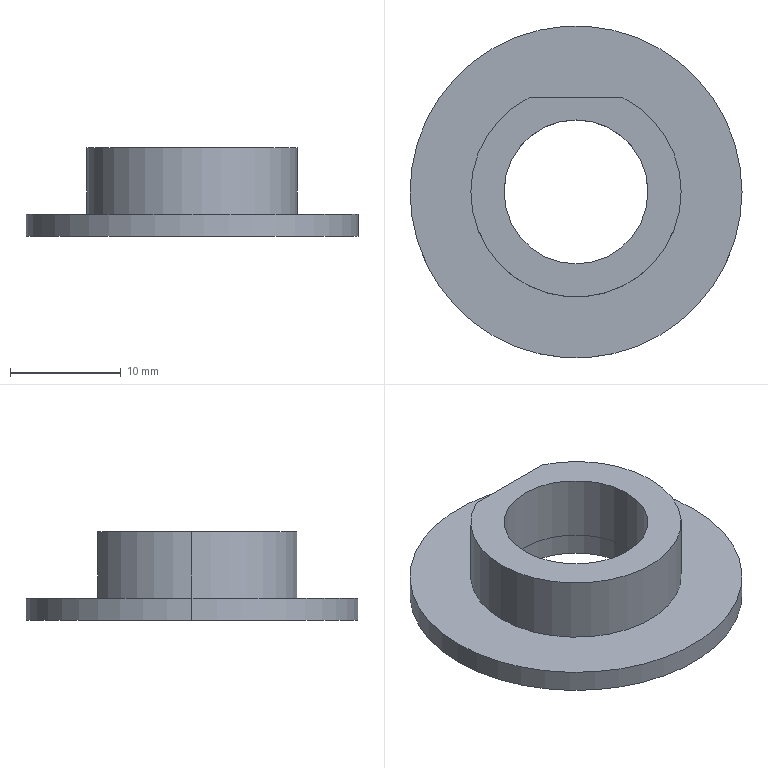Part | SolidWorks | features ICE 3, Extrusion 1 | 2 solids | 14 faces | box 30 x 30 x 8 mm | volume 2019 mm3 | cylinder 9 | plane 5 | commonest cylinder face diameters 13 x4 19 x3 30 x2
STEP:
#1=CARTESIAN_POINT('',(-6.5,0.,0.));
#2=VERTEX_POINT('',#1);
#3=CARTESIAN_POINT('',(6.5,0.,0.));
#4=VERTEX_POINT('',#3);
#5=CARTESIAN_POINT('',(0.,0.,0.));
#6=DIRECTION('',(0.,0.,1.));
#7=DIRECTION('',(1.,0.,0.));
#8=AXIS2_PLACEMENT_3D('',#5,#6,#7);
#9=CIRCLE('',#8,6.5);
#10=EDGE_CURVE('',#2,#4,#9,.T.);
#11=ORIENTED_EDGE('',*,*,#10,.F.);
#12=CARTESIAN_POINT('',(-6.5,0.,2.));
#13=VERTEX_POINT('',#12);
#14=CARTESIAN_POINT('',(-6.5,0.,-7.));
#15=DIRECTION('',(0.,0.,1.));
#16=VECTOR('',#15,1000.);
#17=LINE('',#14,#16);
#18=EDGE_CURVE('',#2,#13,#17,.T.);
#19=ORIENTED_EDGE('',*,*,#18,.T.);
#20=CARTESIAN_POINT('',(6.5,0.,2.));
#21=VERTEX_POINT('',#20);
#22=CARTESIAN_POINT('',(0.,0.,2.));
#23=DIRECTION('',(0.,0.,1.));
#24=DIRECTION('',(1.,0.,0.));
#25=AXIS2_PLACEMENT_3D('',#22,#23,#24);
#26=CIRCLE('',#25,6.5);
#27=EDGE_CURVE('',#13,#21,#26,.T.);
#28=ORIENTED_EDGE('',*,*,#27,.T.);
#29=CARTESIAN_POINT('',(6.5,0.,-7.));
#30=DIRECTION('',(0.,0.,1.));
#31=VECTOR('',#30,1000.);
#32=LINE('',#29,#31);
#33=EDGE_CURVE('',#4,#21,#32,.T.);
#34=ORIENTED_EDGE('',*,*,#33,.F.);
#35=EDGE_LOOP('',(#11,#19,#28,#34));
#36=FACE_OUTER_BOUND('',#35,.T.);
#37=CARTESIAN_POINT('',(0.,0.,-7.));
#38=DIRECTION('',(0.,0.,1.));
#39=DIRECTION('',(1.,0.,0.));
#40=AXIS2_PLACEMENT_3D('',#37,#38,#39);
#41=CYLINDRICAL_SURFACE('',#40,6.5);
#42=ADVANCED_FACE('',(#36),#41,.F.);
#43=CARTESIAN_POINT('',(15.,0.,2.));
#44=VERTEX_POINT('',#43);
#45=CARTESIAN_POINT('',(-15.,0.,2.));
#46=VERTEX_POINT('',#45);
#47=CARTESIAN_POINT('',(0.,0.,2.));
#48=DIRECTION('',(0.,0.,1.));
#49=DIRECTION('',(1.,0.,0.));
#50=AXIS2_PLACEMENT_3D('',#47,#48,#49);
#51=CIRCLE('',#50,15.);
#52=EDGE_CURVE('',#44,#46,#51,.T.);
#53=ORIENTED_EDGE('',*,*,#52,.F.);
#54=CARTESIAN_POINT('',(15.,0.,0.));
#55=VERTEX_POINT('',#54);
#56=CARTESIAN_POINT('',(15.,0.,2.));
#57=DIRECTION('',(0.,0.,-1.));
#58=VECTOR('',#57,1000.);
#59=LINE('',#56,#58);
#60=EDGE_CURVE('',#44,#55,#59,.T.);
#61=ORIENTED_EDGE('',*,*,#60,.T.);
#62=CARTESIAN_POINT('',(-15.,0.,0.));
#63=VERTEX_POINT('',#62);
#64=CARTESIAN_POINT('',(0.,0.,0.));
#65=DIRECTION('',(0.,0.,1.));
#66=DIRECTION('',(1.,0.,0.));
#67=AXIS2_PLACEMENT_3D('',#64,#65,#66);
#68=CIRCLE('',#67,15.);
#69=EDGE_CURVE('',#55,#63,#68,.T.);
#70=ORIENTED_EDGE('',*,*,#69,.T.);
#71=CARTESIAN_POINT('',(-15.,0.,2.));
#72=DIRECTION('',(0.,0.,-1.));
#73=VECTOR('',#72,1000.);
#74=LINE('',#71,#73);
#75=EDGE_CURVE('',#46,#63,#74,.T.);
#76=ORIENTED_EDGE('',*,*,#75,.F.);
#77=EDGE_LOOP('',(#53,#61,#70,#76));
#78=FACE_OUTER_BOUND('',#77,.T.);
#79=CARTESIAN_POINT('',(0.,0.,2.));
#80=DIRECTION('',(0.,0.,-1.));
#81=DIRECTION('',(-1.,0.,0.));
#82=AXIS2_PLACEMENT_3D('',#79,#80,#81);
#83=CYLINDRICAL_SURFACE('',#82,15.);
#84=ADVANCED_FACE('',(#78),#83,.T.);
#85=ORIENTED_EDGE('',*,*,#60,.F.);
#86=CARTESIAN_POINT('',(0.,0.,2.));
#87=DIRECTION('',(0.,0.,1.));
#88=DIRECTION('',(1.,0.,0.));
#89=AXIS2_PLACEMENT_3D('',#86,#87,#88);
#90=CIRCLE('',#89,15.);
#91=EDGE_CURVE('',#46,#44,#90,.T.);
#92=ORIENTED_EDGE('',*,*,#91,.F.);
#93=ORIENTED_EDGE('',*,*,#75,.T.);
#94=CARTESIAN_POINT('',(0.,0.,0.));
#95=DIRECTION('',(0.,0.,1.));
#96=DIRECTION('',(1.,0.,0.));
#97=AXIS2_PLACEMENT_3D('',#94,#95,#96);
#98=CIRCLE('',#97,15.);
#99=EDGE_CURVE('',#63,#55,#98,.T.);
#100=ORIENTED_EDGE('',*,*,#99,.T.);
#101=EDGE_LOOP('',(#85,#92,#93,#100));
#102=FACE_OUTER_BOUND('',#101,.T.);
#103=CARTESIAN_POINT('',(0.,0.,2.));
#104=DIRECTION('',(0.,0.,-1.));
#105=DIRECTION('',(-1.,0.,0.));
#106=AXIS2_PLACEMENT_3D('',#103,#104,#105);
#107=CYLINDRICAL_SURFACE('',#106,15.);
#108=ADVANCED_FACE('',(#102),#107,.T.);
#109=CARTESIAN_POINT('',(0.,0.,2.));
#110=DIRECTION('',(0.,0.,1.));
#111=DIRECTION('',(1.,0.,0.));
#112=AXIS2_PLACEMENT_3D('',#109,#110,#111);
#113=CIRCLE('',#112,6.5);
#114=EDGE_CURVE('',#21,#13,#113,.T.);
#115=ORIENTED_EDGE('',*,*,#114,.F.);
#116=ORIENTED_EDGE('',*,*,#27,.F.);
#117=EDGE_LOOP('',(#115,#116));
#118=FACE_BOUND('',#117,.T.);
#119=ORIENTED_EDGE('',*,*,#91,.T.);
#120=ORIENTED_EDGE('',*,*,#52,.T.);
#121=EDGE_LOOP('',(#119,#120));
#122=FACE_OUTER_BOUND('',#121,.T.);
#123=CARTESIAN_POINT('',(0.,0.,2.));
#124=DIRECTION('',(0.,0.,1.));
#125=DIRECTION('',(1.,0.,0.));
#126=AXIS2_PLACEMENT_3D('',#123,#124,#125);
#127=PLANE('',#126);
#128=ADVANCED_FACE('',(#118,#122),#127,.T.);
#129=CARTESIAN_POINT('',(0.,0.,0.));
#130=DIRECTION('',(0.,0.,1.));
#131=DIRECTION('',(1.,0.,0.));
#132=AXIS2_PLACEMENT_3D('',#129,#130,#131);
#133=CIRCLE('',#132,6.5);
#134=EDGE_CURVE('',#4,#2,#133,.T.);
#135=ORIENTED_EDGE('',*,*,#134,.T.);
#136=ORIENTED_EDGE('',*,*,#10,.T.);
#137=EDGE_LOOP('',(#135,#136));
#138=FACE_BOUND('',#137,.T.);
#139=ORIENTED_EDGE('',*,*,#99,.F.);
#140=ORIENTED_EDGE('',*,*,#69,.F.);
#141=EDGE_LOOP('',(#139,#140));
#142=FACE_OUTER_BOUND('',#141,.T.);
#143=CARTESIAN_POINT('',(0.,0.,0.));
#144=DIRECTION('',(0.,0.,1.));
#145=DIRECTION('',(1.,0.,0.));
#146=AXIS2_PLACEMENT_3D('',#143,#144,#145);
#147=PLANE('',#146);
#148=ADVANCED_FACE('',(#138,#142),#147,.F.);
#149=ORIENTED_EDGE('',*,*,#18,.F.);
#150=ORIENTED_EDGE('',*,*,#134,.F.);
#151=ORIENTED_EDGE('',*,*,#33,.T.);
#152=ORIENTED_EDGE('',*,*,#114,.T.);
#153=EDGE_LOOP('',(#149,#150,#151,#152));
#154=FACE_OUTER_BOUND('',#153,.T.);
#155=CARTESIAN_POINT('',(0.,0.,-7.));
#156=DIRECTION('',(0.,0.,1.));
#157=DIRECTION('',(1.,0.,0.));
#158=AXIS2_PLACEMENT_3D('',#155,#156,#157);
#159=CYLINDRICAL_SURFACE('',#158,6.5);
#160=ADVANCED_FACE('',(#154),#159,.F.);
#161=CLOSED_SHELL('',(#42,#84,#108,#128,#148,#160));
#162=MANIFOLD_SOLID_BREP('',#161);
#163=CARTESIAN_POINT('',(-6.5,0.,2.));
#164=VERTEX_POINT('',#163);
#165=CARTESIAN_POINT('',(6.5,0.,2.));
#166=VERTEX_POINT('',#165);
#167=CARTESIAN_POINT('',(0.,0.,2.));
#168=DIRECTION('',(0.,0.,1.));
#169=DIRECTION('',(1.,0.,0.));
#170=AXIS2_PLACEMENT_3D('',#167,#168,#169);
#171=CIRCLE('',#170,6.5);
#172=EDGE_CURVE('',#164,#166,#171,.T.);
#173=ORIENTED_EDGE('',*,*,#172,.F.);
#174=CARTESIAN_POINT('',(-6.5,0.,8.));
#175=VERTEX_POINT('',#174);
#176=CARTESIAN_POINT('',(-6.5,0.,-7.));
#177=DIRECTION('',(0.,0.,1.));
#178=VECTOR('',#177,1000.);
#179=LINE('',#176,#178);
#180=EDGE_CURVE('',#164,#175,#179,.T.);
#181=ORIENTED_EDGE('',*,*,#180,.T.);
#182=CARTESIAN_POINT('',(6.5,0.,8.));
#183=VERTEX_POINT('',#182);
#184=CARTESIAN_POINT('',(0.,0.,8.));
#185=DIRECTION('',(0.,0.,1.));
#186=DIRECTION('',(1.,0.,0.));
#187=AXIS2_PLACEMENT_3D('',#184,#185,#186);
#188=CIRCLE('',#187,6.5);
#189=EDGE_CURVE('',#175,#183,#188,.T.);
#190=ORIENTED_EDGE('',*,*,#189,.T.);
#191=CARTESIAN_POINT('',(6.5,0.,-7.));
#192=DIRECTION('',(0.,0.,1.));
#193=VECTOR('',#192,1000.);
#194=LINE('',#191,#193);
#195=EDGE_CURVE('',#166,#183,#194,.T.);
#196=ORIENTED_EDGE('',*,*,#195,.F.);
#197=EDGE_LOOP('',(#173,#181,#190,#196));
#198=FACE_OUTER_BOUND('',#197,.T.);
#199=CARTESIAN_POINT('',(0.,0.,-7.));
#200=DIRECTION('',(0.,0.,1.));
#201=DIRECTION('',(1.,0.,0.));
#202=AXIS2_PLACEMENT_3D('',#199,#200,#201);
#203=CYLINDRICAL_SURFACE('',#202,6.5);
#204=ADVANCED_FACE('',(#198),#203,.F.);
#205=CARTESIAN_POINT('',(9.5,0.,8.));
#206=VERTEX_POINT('',#205);
#207=CARTESIAN_POINT('',(4.243,8.5,8.));
#208=VERTEX_POINT('',#207);
#209=CARTESIAN_POINT('',(0.,0.,8.));
#210=DIRECTION('',(0.,0.,1.));
#211=DIRECTION('',(1.,0.,0.));
#212=AXIS2_PLACEMENT_3D('',#209,#210,#211);
#213=CIRCLE('',#212,9.5);
#214=EDGE_CURVE('',#206,#208,#213,.T.);
#215=ORIENTED_EDGE('',*,*,#214,.F.);
#216=CARTESIAN_POINT('',(9.5,0.,2.));
#217=VERTEX_POINT('',#216);
#218=CARTESIAN_POINT('',(9.5,0.,8.));
#219=DIRECTION('',(0.,0.,-1.));
#220=VECTOR('',#219,1000.);
#221=LINE('',#218,#220);
#222=EDGE_CURVE('',#206,#217,#221,.T.);
#223=ORIENTED_EDGE('',*,*,#222,.T.);
#224=CARTESIAN_POINT('',(4.243,8.5,2.));
#225=VERTEX_POINT('',#224);
#226=CARTESIAN_POINT('',(0.,0.,2.));
#227=DIRECTION('',(0.,0.,1.));
#228=DIRECTION('',(1.,0.,0.));
#229=AXIS2_PLACEMENT_3D('',#226,#227,#228);
#230=CIRCLE('',#229,9.5);
#231=EDGE_CURVE('',#217,#225,#230,.T.);
#232=ORIENTED_EDGE('',*,*,#231,.T.);
#233=CARTESIAN_POINT('',(4.243,8.5,-6.544));
#234=DIRECTION('',(0.,0.,1.));
#235=VECTOR('',#234,1000.);
#236=LINE('',#233,#235);
#237=EDGE_CURVE('',#225,#208,#236,.T.);
#238=ORIENTED_EDGE('',*,*,#237,.T.);
#239=EDGE_LOOP('',(#215,#223,#232,#238));
#240=FACE_OUTER_BOUND('',#239,.T.);
#241=CARTESIAN_POINT('',(0.,0.,8.));
#242=DIRECTION('',(0.,0.,-1.));
#243=DIRECTION('',(-1.,0.,0.));
#244=AXIS2_PLACEMENT_3D('',#241,#242,#243);
#245=CYLINDRICAL_SURFACE('',#244,9.5);
#246=ADVANCED_FACE('',(#240),#245,.T.);
#247=ORIENTED_EDGE('',*,*,#222,.F.);
#248=CARTESIAN_POINT('',(-9.5,0.,8.));
#249=VERTEX_POINT('',#248);
#250=CARTESIAN_POINT('',(0.,0.,8.));
#251=DIRECTION('',(0.,0.,1.));
#252=DIRECTION('',(1.,0.,0.));
#253=AXIS2_PLACEMENT_3D('',#250,#251,#252);
#254=CIRCLE('',#253,9.5);
#255=EDGE_CURVE('',#249,#206,#254,.T.);
#256=ORIENTED_EDGE('',*,*,#255,.F.);
#257=CARTESIAN_POINT('',(-9.5,0.,2.));
#258=VERTEX_POINT('',#257);
#259=CARTESIAN_POINT('',(-9.5,0.,8.));
#260=DIRECTION('',(0.,0.,-1.));
#261=VECTOR('',#260,1000.);
#262=LINE('',#259,#261);
#263=EDGE_CURVE('',#249,#258,#262,.T.);
#264=ORIENTED_EDGE('',*,*,#263,.T.);
#265=CARTESIAN_POINT('',(0.,0.,2.));
#266=DIRECTION('',(0.,0.,1.));
#267=DIRECTION('',(1.,0.,0.));
#268=AXIS2_PLACEMENT_3D('',#265,#266,#267);
#269=CIRCLE('',#268,9.5);
#270=EDGE_CURVE('',#258,#217,#269,.T.);
#271=ORIENTED_EDGE('',*,*,#270,.T.);
#272=EDGE_LOOP('',(#247,#256,#264,#271));
#273=FACE_OUTER_BOUND('',#272,.T.);
#274=CARTESIAN_POINT('',(0.,0.,8.));
#275=DIRECTION('',(0.,0.,-1.));
#276=DIRECTION('',(-1.,0.,0.));
#277=AXIS2_PLACEMENT_3D('',#274,#275,#276);
#278=CYLINDRICAL_SURFACE('',#277,9.5);
#279=ADVANCED_FACE('',(#273),#278,.T.);
#280=ORIENTED_EDGE('',*,*,#263,.F.);
#281=CARTESIAN_POINT('',(-4.243,8.5,8.));
#282=VERTEX_POINT('',#281);
#283=CARTESIAN_POINT('',(0.,0.,8.));
#284=DIRECTION('',(0.,0.,1.));
#285=DIRECTION('',(1.,0.,0.));
#286=AXIS2_PLACEMENT_3D('',#283,#284,#285);
#287=CIRCLE('',#286,9.5);
#288=EDGE_CURVE('',#282,#249,#287,.T.);
#289=ORIENTED_EDGE('',*,*,#288,.F.);
#290=CARTESIAN_POINT('',(-4.243,8.5,2.));
#291=VERTEX_POINT('',#290);
#292=CARTESIAN_POINT('',(-4.243,8.5,-6.544));
#293=DIRECTION('',(0.,0.,1.));
#294=VECTOR('',#293,1000.);
#295=LINE('',#292,#294);
#296=EDGE_CURVE('',#291,#282,#295,.T.);
#297=ORIENTED_EDGE('',*,*,#296,.F.);
#298=CARTESIAN_POINT('',(0.,0.,2.));
#299=DIRECTION('',(0.,0.,1.));
#300=DIRECTION('',(1.,0.,0.));
#301=AXIS2_PLACEMENT_3D('',#298,#299,#300);
#302=CIRCLE('',#301,9.5);
#303=EDGE_CURVE('',#291,#258,#302,.T.);
#304=ORIENTED_EDGE('',*,*,#303,.T.);
#305=EDGE_LOOP('',(#280,#289,#297,#304));
#306=FACE_OUTER_BOUND('',#305,.T.);
#307=CARTESIAN_POINT('',(0.,0.,8.));
#308=DIRECTION('',(0.,0.,-1.));
#309=DIRECTION('',(-1.,0.,0.));
#310=AXIS2_PLACEMENT_3D('',#307,#308,#309);
#311=CYLINDRICAL_SURFACE('',#310,9.5);
#312=ADVANCED_FACE('',(#306),#311,.T.);
#313=CARTESIAN_POINT('',(-4.243,8.5,8.));
#314=DIRECTION('',(1.,0.,0.));
#315=VECTOR('',#314,1000.);
#316=LINE('',#313,#315);
#317=EDGE_CURVE('',#282,#208,#316,.T.);
#318=ORIENTED_EDGE('',*,*,#317,.F.);
#319=ORIENTED_EDGE('',*,*,#288,.T.);
#320=ORIENTED_EDGE('',*,*,#255,.T.);
#321=ORIENTED_EDGE('',*,*,#214,.T.);
#322=EDGE_LOOP('',(#318,#319,#320,#321));
#323=FACE_OUTER_BOUND('',#322,.T.);
#324=CARTESIAN_POINT('',(0.,0.,8.));
#325=DIRECTION('',(0.,0.,1.));
#326=DIRECTION('',(1.,0.,0.));
#327=AXIS2_PLACEMENT_3D('',#324,#325,#326);
#328=CIRCLE('',#327,6.5);
#329=EDGE_CURVE('',#183,#175,#328,.T.);
#330=ORIENTED_EDGE('',*,*,#329,.F.);
#331=ORIENTED_EDGE('',*,*,#189,.F.);
#332=EDGE_LOOP('',(#330,#331));
#333=FACE_BOUND('',#332,.T.);
#334=CARTESIAN_POINT('',(0.,0.,8.));
#335=DIRECTION('',(0.,0.,1.));
#336=DIRECTION('',(1.,0.,0.));
#337=AXIS2_PLACEMENT_3D('',#334,#335,#336);
#338=PLANE('',#337);
#339=ADVANCED_FACE('',(#323,#333),#338,.T.);
#340=CARTESIAN_POINT('',(0.,0.,2.));
#341=DIRECTION('',(0.,0.,1.));
#342=DIRECTION('',(1.,0.,0.));
#343=AXIS2_PLACEMENT_3D('',#340,#341,#342);
#344=CIRCLE('',#343,6.5);
#345=EDGE_CURVE('',#166,#164,#344,.T.);
#346=ORIENTED_EDGE('',*,*,#345,.T.);
#347=ORIENTED_EDGE('',*,*,#172,.T.);
#348=EDGE_LOOP('',(#346,#347));
#349=FACE_BOUND('',#348,.T.);
#350=ORIENTED_EDGE('',*,*,#303,.F.);
#351=CARTESIAN_POINT('',(-4.243,8.5,2.));
#352=DIRECTION('',(-1.,0.,0.));
#353=VECTOR('',#352,1000.);
#354=LINE('',#351,#353);
#355=EDGE_CURVE('',#225,#291,#354,.T.);
#356=ORIENTED_EDGE('',*,*,#355,.F.);
#357=ORIENTED_EDGE('',*,*,#231,.F.);
#358=ORIENTED_EDGE('',*,*,#270,.F.);
#359=EDGE_LOOP('',(#350,#356,#357,#358));
#360=FACE_OUTER_BOUND('',#359,.T.);
#361=CARTESIAN_POINT('',(0.,0.,2.));
#362=DIRECTION('',(0.,0.,1.));
#363=DIRECTION('',(1.,0.,0.));
#364=AXIS2_PLACEMENT_3D('',#361,#362,#363);
#365=PLANE('',#364);
#366=ADVANCED_FACE('',(#349,#360),#365,.F.);
#367=ORIENTED_EDGE('',*,*,#180,.F.);
#368=ORIENTED_EDGE('',*,*,#345,.F.);
#369=ORIENTED_EDGE('',*,*,#195,.T.);
#370=ORIENTED_EDGE('',*,*,#329,.T.);
#371=EDGE_LOOP('',(#367,#368,#369,#370));
#372=FACE_OUTER_BOUND('',#371,.T.);
#373=CARTESIAN_POINT('',(0.,0.,-7.));
#374=DIRECTION('',(0.,0.,1.));
#375=DIRECTION('',(1.,0.,0.));
#376=AXIS2_PLACEMENT_3D('',#373,#374,#375);
#377=CYLINDRICAL_SURFACE('',#376,6.5);
#378=ADVANCED_FACE('',(#372),#377,.F.);
#379=ORIENTED_EDGE('',*,*,#355,.T.);
#380=ORIENTED_EDGE('',*,*,#296,.T.);
#381=ORIENTED_EDGE('',*,*,#317,.T.);
#382=ORIENTED_EDGE('',*,*,#237,.F.);
#383=EDGE_LOOP('',(#379,#380,#381,#382));
#384=FACE_OUTER_BOUND('',#383,.T.);
#385=CARTESIAN_POINT('',(-4.243,8.5,-6.544));
#386=DIRECTION('',(0.,-1.,0.));
#387=DIRECTION('',(0.,0.,-1.));
#388=AXIS2_PLACEMENT_3D('',#385,#386,#387);
#389=PLANE('',#388);
#390=ADVANCED_FACE('',(#384),#389,.F.);
#391=CLOSED_SHELL('',(#204,#246,#279,#312,#339,#366,#378,#390));
#392=MANIFOLD_SOLID_BREP('',#391);
#393=CARTESIAN_POINT('',(0.,0.,0.));
#394=DIRECTION('',(0.,0.,1.));
#395=DIRECTION('',(1.,0.,0.));
#396=AXIS2_PLACEMENT_3D('',#393,#394,#395);
#397=(LENGTH_UNIT()NAMED_UNIT(*)SI_UNIT(.MILLI.,.METRE.));
#398=UNCERTAINTY_MEASURE_WITH_UNIT(LENGTH_MEASURE(0.00001),#397,'','');
#399=(NAMED_UNIT(*)PLANE_ANGLE_UNIT()SI_UNIT($,.RADIAN.));
#400=(NAMED_UNIT(*)SI_UNIT($,.STERADIAN.)SOLID_ANGLE_UNIT());
#401=(GEOMETRIC_REPRESENTATION_CONTEXT(3)GLOBAL_UNCERTAINTY_ASSIGNED_CONTEXT((#398))GLOBAL_UNIT_ASSIGNED_CONTEXT((#397,#399,#400))REPRESENTATION_CONTEXT('',''));
#402=ADVANCED_BREP_SHAPE_REPRESENTATION('',(#162,#392,#396),#401);